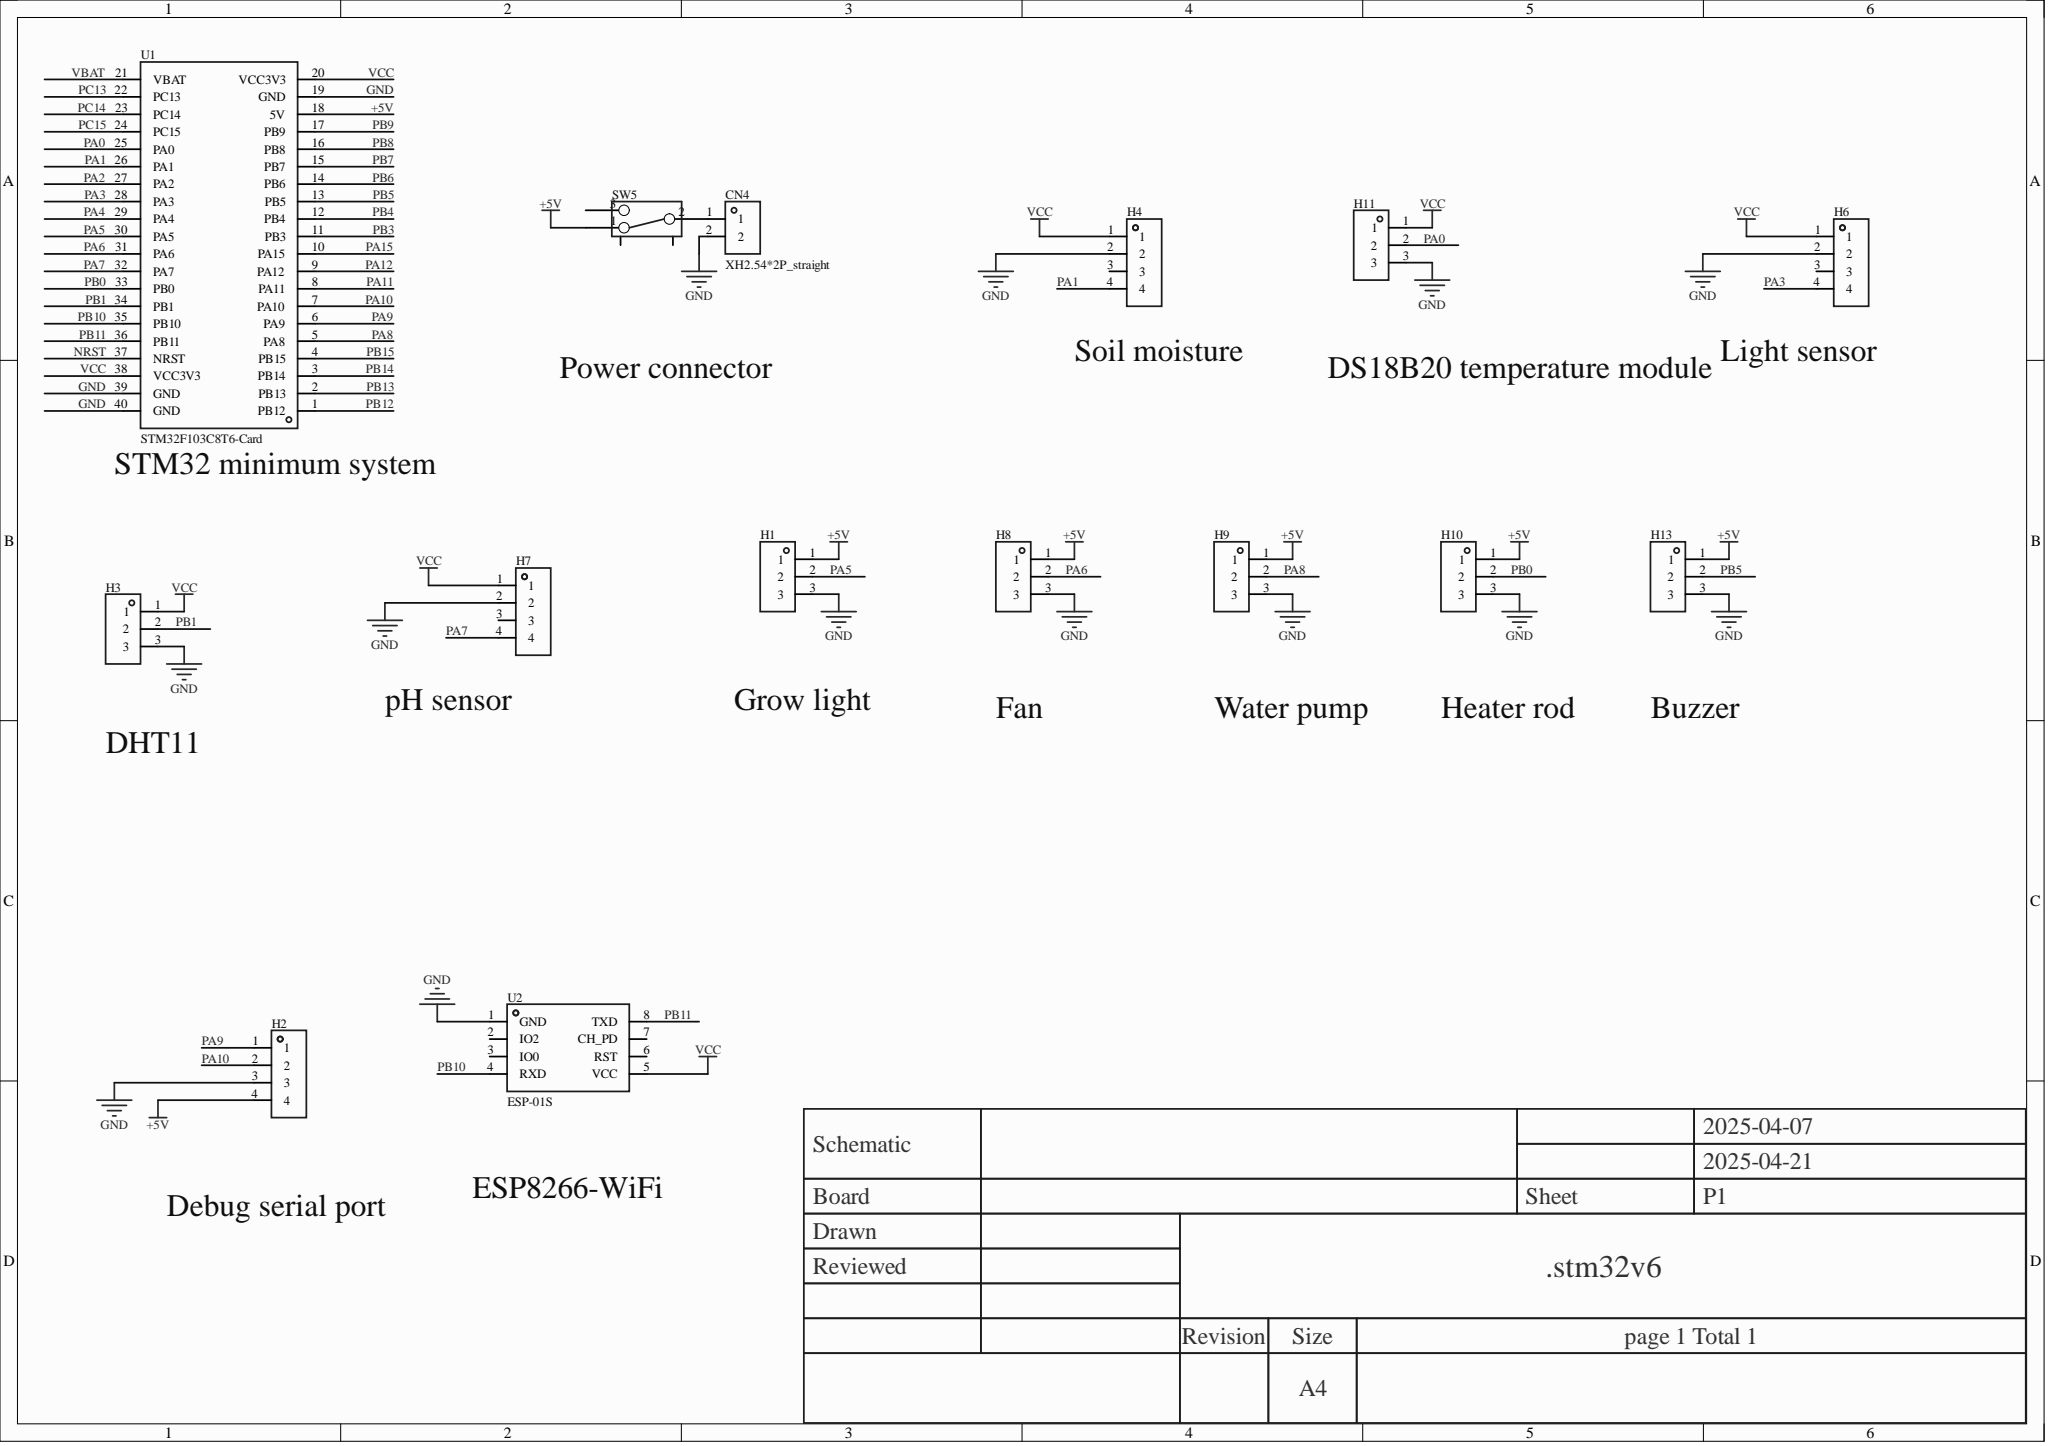Circuit board | Altium Designer | 15 parts | 18 nets
Bill of materials:
Comment,Description,Designator,Footprint,LibRef,Quantity
"XH2.54*2P_straight","","CN4","CONN-TH_2P-P2.50-XH2.54-2P","XH2.54*2P_直插","1"
"","","H1, H3, H8, H9, H10, H11, H13","HDR-TH_3P-P2.54-V-F","HDR-F_2.54_1x3P","7"
"","","H2, H4, H6, H7","HDR-TH_4P-P2.54-V-F","HDR-F_2.54_1x4P","4"
"","","SW5","拨动开关","拨动开关_正","1"
"STM32F103C8T6-Card","","U1","CONN-TH_L53.3-W22.9_STM32F103C8T6-CARD","STM32F103C8T6-Card","1"
"ESP-01S","","U2","WIFIM-TH_ESP-01S","ESP-01S_C111009","1"
Netlist (Protel format):
[
CN4
CONN-TH_2P-P2.50-XH2.54-2P
XH2.54*2P_straight



]
[
H1
HDR-TH_3P-P2.54-V-F




]
[
H2
HDR-TH_4P-P2.54-V-F




]
[
H3
HDR-TH_3P-P2.54-V-F




]
[
H4
HDR-TH_4P-P2.54-V-F




]
[
H6
HDR-TH_4P-P2.54-V-F




]
[
H7
HDR-TH_4P-P2.54-V-F




]
[
H8
HDR-TH_3P-P2.54-V-F




]
[
H9
HDR-TH_3P-P2.54-V-F




]
[
H10
HDR-TH_3P-P2.54-V-F




]
[
H11
HDR-TH_3P-P2.54-V-F




]
[
H13
HDR-TH_3P-P2.54-V-F




]
[
SW5
拨动开关




]
[
U1
CONN-TH_L53.3-W22.9_STM32F103C8T6-CARD
STM32F103C8T6-Card



]
[
U2
WIFIM-TH_ESP-01S
ESP-01S



]
(
VCC
H3-1
H4-1
H6-1
H7-1
H11-1
U1-20
U1-38
U2-5
)
(
PB11
U1-36
U2-8
)
(
PB10
U1-35
U2-4
)
(
PB5
H13-2
U1-13
)
(
PB1
H3-2
U1-34
)
(
PB0
H10-2
U1-33
)
(
PA10
H2-2
U1-7
)
(
PA9
H2-1
U1-6
)
(
PA8
H9-2
U1-5
)
(
PA7
H7-4
U1-32
)
(
PA6
H8-2
U1-31
)
(
PA5
H1-2
U1-30
)
(
PA3
H6-4
U1-28
)
(
PA1
H4-4
U1-26
)
(
PA0
H11-2
U1-25
)
(
NetCN4_1
CN4-1
SW5-2
)
(
GND
CN4-2
H1-3
H2-3
H3-3
H4-2
H6-2
H7-2
H8-3
H9-3
H10-3
H11-3
H13-3
U1-19
U1-39
U1-40
U2-1
)
(
+5V
H1-1
H2-4
H8-1
H9-1
H10-1
H13-1
SW5-1
U1-18
)